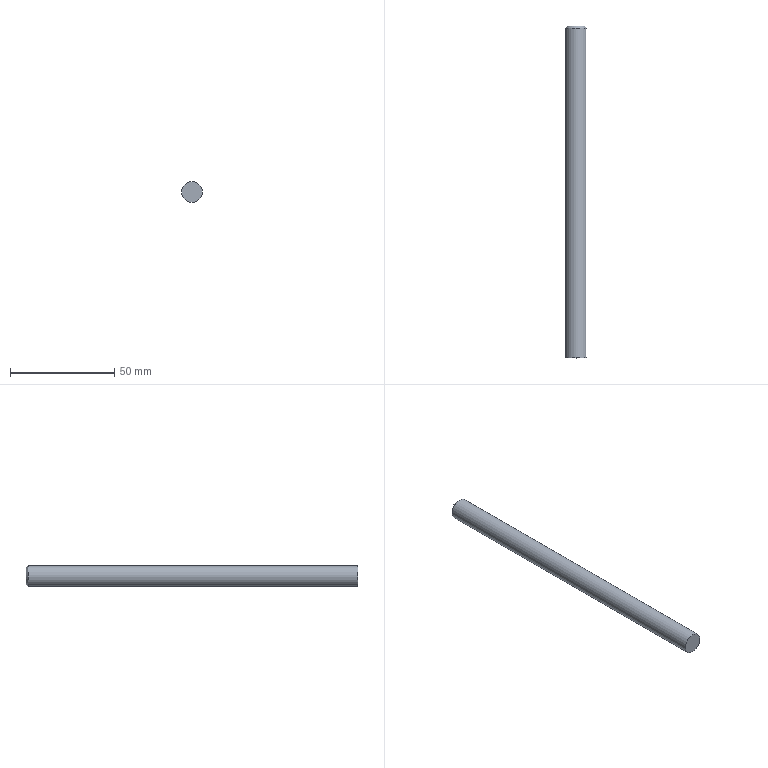Part | NX | features WGN01-25-100-Y-2-002 2 | 1 solid | 4 faces | box 10 x 159.55 x 10 mm | volume 12516 mm3 | plane 2 | cylinder 1 | cone 1 | commonest cylinder face diameters 10 x1
STEP:
#1=CARTESIAN_POINT('',(0.000006093,201.666,168.366));
#2=VERTEX_POINT('',#1);
#3=CARTESIAN_POINT('',(0.000006093,201.666,173.366));
#4=DIRECTION('',(0.,-1.,0.));
#5=DIRECTION('',(0.,0.,-1.));
#6=AXIS2_PLACEMENT_3D('',#3,#4,#5);
#7=CIRCLE('',#6,5.);
#8=EDGE_CURVE('',#2,#2,#7,.F.);
#9=ORIENTED_EDGE('',*,*,#8,.F.);
#10=EDGE_LOOP('',(#9));
#11=FACE_BOUND('',#10,.T.);
#12=CARTESIAN_POINT('',(-0.000001192,201.666,111.866));
#13=DIRECTION('',(0.,-1.,0.));
#14=DIRECTION('',(1.,0.,-0.000000009));
#15=AXIS2_PLACEMENT_3D('',#12,#13,#14);
#16=PLANE('',#15);
#17=ADVANCED_FACE('',(#11),#16,.T.);
#18=CARTESIAN_POINT('',(0.000006093,360.216,168.366));
#19=VERTEX_POINT('',#18);
#20=CARTESIAN_POINT('',(0.000006093,360.216,173.366));
#21=DIRECTION('',(0.,-1.,0.));
#22=DIRECTION('',(0.,0.,-1.));
#23=AXIS2_PLACEMENT_3D('',#20,#21,#22);
#24=CIRCLE('',#23,5.);
#25=EDGE_CURVE('',#19,#19,#24,.T.);
#26=ORIENTED_EDGE('',*,*,#25,.T.);
#27=EDGE_LOOP('',(#26));
#28=FACE_BOUND('',#27,.T.);
#29=ORIENTED_EDGE('',*,*,#8,.T.);
#30=EDGE_LOOP('',(#29));
#31=FACE_BOUND('',#30,.T.);
#32=CARTESIAN_POINT('',(0.000006093,412.332,173.366));
#33=DIRECTION('',(0.,1.,0.));
#34=DIRECTION('',(0.8321,0.,-0.5546));
#35=AXIS2_PLACEMENT_3D('',#32,#33,#34);
#36=CYLINDRICAL_SURFACE('',#35,5.);
#37=ADVANCED_FACE('',(#28,#31),#36,.T.);
#38=CARTESIAN_POINT('',(0.000006093,361.216,177.366));
#39=VERTEX_POINT('',#38);
#40=CARTESIAN_POINT('',(0.000006093,361.216,173.366));
#41=DIRECTION('',(0.,1.,0.));
#42=DIRECTION('',(0.,0.,1.));
#43=AXIS2_PLACEMENT_3D('',#40,#41,#42);
#44=CIRCLE('',#43,4.);
#45=EDGE_CURVE('',#39,#39,#44,.T.);
#46=ORIENTED_EDGE('',*,*,#45,.T.);
#47=EDGE_LOOP('',(#46));
#48=FACE_BOUND('',#47,.T.);
#49=CARTESIAN_POINT('',(-0.000000942,361.216,122.381));
#50=DIRECTION('',(0.,1.,0.));
#51=DIRECTION('',(1.,0.,0.));
#52=AXIS2_PLACEMENT_3D('',#49,#50,#51);
#53=PLANE('',#52);
#54=ADVANCED_FACE('',(#48),#53,.T.);
#55=ORIENTED_EDGE('',*,*,#25,.F.);
#56=EDGE_LOOP('',(#55));
#57=FACE_BOUND('',#56,.T.);
#58=ORIENTED_EDGE('',*,*,#45,.F.);
#59=EDGE_LOOP('',(#58));
#60=FACE_BOUND('',#59,.T.);
#61=CARTESIAN_POINT('',(0.000006093,361.216,173.366));
#62=DIRECTION('',(0.,-1.,0.));
#63=DIRECTION('',(0.,0.,-1.));
#64=AXIS2_PLACEMENT_3D('',#61,#62,#63);
#65=CONICAL_SURFACE('',#64,4.,0.7854);
#66=ADVANCED_FACE('',(#57,#60),#65,.T.);
#67=CLOSED_SHELL('',(#17,#37,#54,#66));
#68=MANIFOLD_SOLID_BREP('',#67);
#69=(LENGTH_UNIT()NAMED_UNIT(*)SI_UNIT(.MILLI.,.METRE.));
#70=UNCERTAINTY_MEASURE_WITH_UNIT(LENGTH_MEASURE(0.00001),#69,'','');
#71=(NAMED_UNIT(*)PLANE_ANGLE_UNIT()SI_UNIT($,.RADIAN.));
#72=(NAMED_UNIT(*)SI_UNIT($,.STERADIAN.)SOLID_ANGLE_UNIT());
#73=(GEOMETRIC_REPRESENTATION_CONTEXT(3)GLOBAL_UNCERTAINTY_ASSIGNED_CONTEXT((#70))GLOBAL_UNIT_ASSIGNED_CONTEXT((#69,#71,#72))REPRESENTATION_CONTEXT('',''));
#74=ADVANCED_BREP_SHAPE_REPRESENTATION('',(#68),#73);